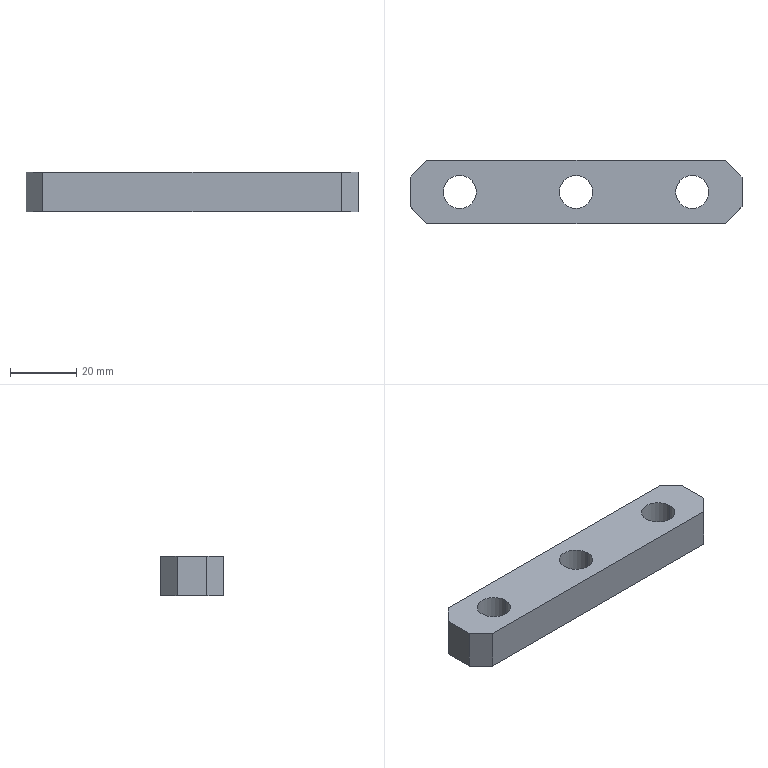Part | STEP file | J453-EBZ05-10-00 | 1 solid | 16 faces | box 100 x 19 x 12 mm | volume 19373 mm3 | plane 10 | cylinder 6 | commonest cylinder face diameters 10 x6
STEP:
#1=CARTESIAN_POINT('',(0.,0.,0.));
#2=DIRECTION('',(0.,0.,1.));
#3=DIRECTION('',(1.,0.,0.));
#4=AXIS2_PLACEMENT_3D('',#1,#2,#3);
#5=CARTESIAN_POINT('',(80.,10.,12.));
#6=VERTEX_POINT('',#5);
#7=CARTESIAN_POINT('',(80.,10.,0.));
#8=VERTEX_POINT('',#7);
#9=CARTESIAN_POINT('',(80.,10.,12.));
#10=DIRECTION('',(0.,0.,-1.));
#11=VECTOR('',#10,1.);
#12=LINE('',#9,#11);
#13=CARTESIAN_POINT('',(85.,10.,12.));
#14=DIRECTION('',(0.,0.,-1.));
#15=DIRECTION('',(-1.,0.,0.));
#16=AXIS2_PLACEMENT_3D('',#13,#14,#15);
#17=CYLINDRICAL_SURFACE('',#16,5.);
#18=CARTESIAN_POINT('',(6.283,0.));
#19=DIRECTION('',(0.,1.));
#20=VECTOR('',#19,1.);
#21=LINE('',#18,#20);
#22=(GEOMETRIC_REPRESENTATION_CONTEXT(2)PARAMETRIC_REPRESENTATION_CONTEXT()REPRESENTATION_CONTEXT('',''));
#23=DEFINITIONAL_REPRESENTATION('',(#21),#22);
#24=PCURVE('',#17,#23);
#25=CARTESIAN_POINT('',(85.,10.,12.));
#26=DIRECTION('',(0.,0.,-1.));
#27=DIRECTION('',(-1.,0.,0.));
#28=AXIS2_PLACEMENT_3D('',#25,#26,#27);
#29=CYLINDRICAL_SURFACE('',#28,5.);
#30=CARTESIAN_POINT('',(0.,0.));
#31=DIRECTION('',(0.,1.));
#32=VECTOR('',#31,1.);
#33=LINE('',#30,#32);
#34=(GEOMETRIC_REPRESENTATION_CONTEXT(2)PARAMETRIC_REPRESENTATION_CONTEXT()REPRESENTATION_CONTEXT('',''));
#35=DEFINITIONAL_REPRESENTATION('',(#33),#34);
#36=PCURVE('',#29,#35);
#37=SURFACE_CURVE('',#12,(#24,#36),.PCURVE_S1.);
#38=EDGE_CURVE('',#6,#8,#37,.T.);
#39=ORIENTED_EDGE('',*,*,#38,.T.);
#40=CARTESIAN_POINT('',(90.,10.,0.));
#41=VERTEX_POINT('',#40);
#42=CARTESIAN_POINT('',(85.,10.,0.));
#43=DIRECTION('',(0.,0.,1.));
#44=DIRECTION('',(1.,0.,0.));
#45=AXIS2_PLACEMENT_3D('',#42,#43,#44);
#46=CIRCLE('',#45,5.);
#47=CARTESIAN_POINT('',(9.425,12.));
#48=DIRECTION('',(-1.,0.));
#49=VECTOR('',#48,1.);
#50=LINE('',#47,#49);
#51=(GEOMETRIC_REPRESENTATION_CONTEXT(2)PARAMETRIC_REPRESENTATION_CONTEXT()REPRESENTATION_CONTEXT('',''));
#52=DEFINITIONAL_REPRESENTATION('',(#50),#51);
#53=PCURVE('',#17,#52);
#54=CARTESIAN_POINT('',(50.,10.,0.00000001));
#55=DIRECTION('',(0.,0.,-1.));
#56=DIRECTION('',(0.,-1.,0.));
#57=AXIS2_PLACEMENT_3D('',#54,#55,#56);
#58=PLANE('',#57);
#59=CARTESIAN_POINT('',(0.,-40.));
#60=CARTESIAN_POINT('',(-8.66,-40.));
#61=CARTESIAN_POINT('',(-4.33,-32.5));
#62=CARTESIAN_POINT('',(0.,-25.));
#63=CARTESIAN_POINT('',(4.33,-32.5));
#64=CARTESIAN_POINT('',(8.66,-40.));
#65=CARTESIAN_POINT('',(0.,-40.));
#66=(BOUNDED_CURVE()B_SPLINE_CURVE(2,(#59,#60,#61,#62,#63,#64,#65),.UNSPECIFIED.,.T.,.F.)B_SPLINE_CURVE_WITH_KNOTS((1,2,2,2,2,1),(-2.094,0.,2.094,4.189,6.283,8.378),.UNSPECIFIED.)CURVE()GEOMETRIC_REPRESENTATION_ITEM()RATIONAL_B_SPLINE_CURVE((1.,0.5,1.,0.5,1.,0.5,1.))REPRESENTATION_ITEM(''));
#67=(GEOMETRIC_REPRESENTATION_CONTEXT(2)PARAMETRIC_REPRESENTATION_CONTEXT()REPRESENTATION_CONTEXT('',''));
#68=DEFINITIONAL_REPRESENTATION('',(#66),#67);
#69=PCURVE('',#58,#68);
#70=SURFACE_CURVE('',#46,(#53,#69),.PCURVE_S1.);
#71=EDGE_CURVE('',#8,#41,#70,.T.);
#72=ORIENTED_EDGE('',*,*,#71,.T.);
#73=CARTESIAN_POINT('',(90.,10.,12.));
#74=VERTEX_POINT('',#73);
#75=CARTESIAN_POINT('',(90.,10.,12.));
#76=DIRECTION('',(0.,0.,-1.));
#77=VECTOR('',#76,1.);
#78=LINE('',#75,#77);
#79=CARTESIAN_POINT('',(3.142,0.));
#80=DIRECTION('',(0.,1.));
#81=VECTOR('',#80,1.);
#82=LINE('',#79,#81);
#83=(GEOMETRIC_REPRESENTATION_CONTEXT(2)PARAMETRIC_REPRESENTATION_CONTEXT()REPRESENTATION_CONTEXT('',''));
#84=DEFINITIONAL_REPRESENTATION('',(#82),#83);
#85=PCURVE('',#17,#84);
#86=CARTESIAN_POINT('',(3.142,0.));
#87=DIRECTION('',(0.,1.));
#88=VECTOR('',#87,1.);
#89=LINE('',#86,#88);
#90=(GEOMETRIC_REPRESENTATION_CONTEXT(2)PARAMETRIC_REPRESENTATION_CONTEXT()REPRESENTATION_CONTEXT('',''));
#91=DEFINITIONAL_REPRESENTATION('',(#89),#90);
#92=PCURVE('',#29,#91);
#93=SURFACE_CURVE('',#78,(#85,#92),.PCURVE_S1.);
#94=EDGE_CURVE('',#74,#41,#93,.T.);
#95=ORIENTED_EDGE('',*,*,#94,.F.);
#96=CARTESIAN_POINT('',(85.,10.,12.));
#97=DIRECTION('',(0.,0.,-1.));
#98=DIRECTION('',(-1.,0.,0.));
#99=AXIS2_PLACEMENT_3D('',#96,#97,#98);
#100=CIRCLE('',#99,5.);
#101=CARTESIAN_POINT('',(0.,0.));
#102=DIRECTION('',(1.,0.));
#103=VECTOR('',#102,1.);
#104=LINE('',#101,#103);
#105=(GEOMETRIC_REPRESENTATION_CONTEXT(2)PARAMETRIC_REPRESENTATION_CONTEXT()REPRESENTATION_CONTEXT('',''));
#106=DEFINITIONAL_REPRESENTATION('',(#104),#105);
#107=PCURVE('',#17,#106);
#108=CARTESIAN_POINT('',(50.,10.,12.));
#109=DIRECTION('',(0.,0.,1.));
#110=DIRECTION('',(0.,1.,0.));
#111=AXIS2_PLACEMENT_3D('',#108,#109,#110);
#112=PLANE('',#111);
#113=CARTESIAN_POINT('',(0.,-30.));
#114=CARTESIAN_POINT('',(8.66,-30.));
#115=CARTESIAN_POINT('',(4.33,-37.5));
#116=CARTESIAN_POINT('',(0.,-45.));
#117=CARTESIAN_POINT('',(-4.33,-37.5));
#118=CARTESIAN_POINT('',(-8.66,-30.));
#119=CARTESIAN_POINT('',(0.,-30.));
#120=(BOUNDED_CURVE()B_SPLINE_CURVE(2,(#113,#114,#115,#116,#117,#118,#119),.UNSPECIFIED.,.T.,.F.)B_SPLINE_CURVE_WITH_KNOTS((1,2,2,2,2,1),(-2.094,0.,2.094,4.189,6.283,8.378),.UNSPECIFIED.)CURVE()GEOMETRIC_REPRESENTATION_ITEM()RATIONAL_B_SPLINE_CURVE((1.,0.5,1.,0.5,1.,0.5,1.))REPRESENTATION_ITEM(''));
#121=(GEOMETRIC_REPRESENTATION_CONTEXT(2)PARAMETRIC_REPRESENTATION_CONTEXT()REPRESENTATION_CONTEXT('',''));
#122=DEFINITIONAL_REPRESENTATION('',(#120),#121);
#123=PCURVE('',#112,#122);
#124=SURFACE_CURVE('',#100,(#107,#123),.PCURVE_S1.);
#125=EDGE_CURVE('',#74,#6,#124,.T.);
#126=ORIENTED_EDGE('',*,*,#125,.T.);
#127=EDGE_LOOP('',(#39,#72,#95,#126));
#128=FACE_BOUND('',#127,.F.);
#129=ADVANCED_FACE('',(#128),#17,.F.);
#130=CARTESIAN_POINT('',(45.,10.,12.));
#131=VERTEX_POINT('',#130);
#132=CARTESIAN_POINT('',(45.,10.,0.));
#133=VERTEX_POINT('',#132);
#134=CARTESIAN_POINT('',(45.,10.,12.));
#135=DIRECTION('',(0.,0.,-1.));
#136=VECTOR('',#135,1.);
#137=LINE('',#134,#136);
#138=CARTESIAN_POINT('',(50.,10.,12.));
#139=DIRECTION('',(0.,0.,-1.));
#140=DIRECTION('',(-1.,0.,0.));
#141=AXIS2_PLACEMENT_3D('',#138,#139,#140);
#142=CYLINDRICAL_SURFACE('',#141,5.);
#143=CARTESIAN_POINT('',(6.283,0.));
#144=DIRECTION('',(0.,1.));
#145=VECTOR('',#144,1.);
#146=LINE('',#143,#145);
#147=(GEOMETRIC_REPRESENTATION_CONTEXT(2)PARAMETRIC_REPRESENTATION_CONTEXT()REPRESENTATION_CONTEXT('',''));
#148=DEFINITIONAL_REPRESENTATION('',(#146),#147);
#149=PCURVE('',#142,#148);
#150=CARTESIAN_POINT('',(50.,10.,12.));
#151=DIRECTION('',(0.,0.,-1.));
#152=DIRECTION('',(-1.,0.,0.));
#153=AXIS2_PLACEMENT_3D('',#150,#151,#152);
#154=CYLINDRICAL_SURFACE('',#153,5.);
#155=CARTESIAN_POINT('',(0.,0.));
#156=DIRECTION('',(0.,1.));
#157=VECTOR('',#156,1.);
#158=LINE('',#155,#157);
#159=(GEOMETRIC_REPRESENTATION_CONTEXT(2)PARAMETRIC_REPRESENTATION_CONTEXT()REPRESENTATION_CONTEXT('',''));
#160=DEFINITIONAL_REPRESENTATION('',(#158),#159);
#161=PCURVE('',#154,#160);
#162=SURFACE_CURVE('',#137,(#149,#161),.PCURVE_S1.);
#163=EDGE_CURVE('',#131,#133,#162,.T.);
#164=ORIENTED_EDGE('',*,*,#163,.T.);
#165=CARTESIAN_POINT('',(55.,10.,0.));
#166=VERTEX_POINT('',#165);
#167=CARTESIAN_POINT('',(50.,10.,0.));
#168=DIRECTION('',(0.,0.,1.));
#169=DIRECTION('',(1.,0.,0.));
#170=AXIS2_PLACEMENT_3D('',#167,#168,#169);
#171=CIRCLE('',#170,5.);
#172=CARTESIAN_POINT('',(9.425,12.));
#173=DIRECTION('',(-1.,0.));
#174=VECTOR('',#173,1.);
#175=LINE('',#172,#174);
#176=(GEOMETRIC_REPRESENTATION_CONTEXT(2)PARAMETRIC_REPRESENTATION_CONTEXT()REPRESENTATION_CONTEXT('',''));
#177=DEFINITIONAL_REPRESENTATION('',(#175),#176);
#178=PCURVE('',#142,#177);
#179=CARTESIAN_POINT('',(0.,-5.));
#180=CARTESIAN_POINT('',(-8.66,-5.));
#181=CARTESIAN_POINT('',(-4.33,2.5));
#182=CARTESIAN_POINT('',(0.,10.));
#183=CARTESIAN_POINT('',(4.33,2.5));
#184=CARTESIAN_POINT('',(8.66,-5.));
#185=CARTESIAN_POINT('',(0.,-5.));
#186=(BOUNDED_CURVE()B_SPLINE_CURVE(2,(#179,#180,#181,#182,#183,#184,#185),.UNSPECIFIED.,.T.,.F.)B_SPLINE_CURVE_WITH_KNOTS((1,2,2,2,2,1),(-2.094,0.,2.094,4.189,6.283,8.378),.UNSPECIFIED.)CURVE()GEOMETRIC_REPRESENTATION_ITEM()RATIONAL_B_SPLINE_CURVE((1.,0.5,1.,0.5,1.,0.5,1.))REPRESENTATION_ITEM(''));
#187=(GEOMETRIC_REPRESENTATION_CONTEXT(2)PARAMETRIC_REPRESENTATION_CONTEXT()REPRESENTATION_CONTEXT('',''));
#188=DEFINITIONAL_REPRESENTATION('',(#186),#187);
#189=PCURVE('',#58,#188);
#190=SURFACE_CURVE('',#171,(#178,#189),.PCURVE_S1.);
#191=EDGE_CURVE('',#133,#166,#190,.T.);
#192=ORIENTED_EDGE('',*,*,#191,.T.);
#193=CARTESIAN_POINT('',(55.,10.,12.));
#194=VERTEX_POINT('',#193);
#195=CARTESIAN_POINT('',(55.,10.,12.));
#196=DIRECTION('',(0.,0.,-1.));
#197=VECTOR('',#196,1.);
#198=LINE('',#195,#197);
#199=CARTESIAN_POINT('',(3.142,0.));
#200=DIRECTION('',(0.,1.));
#201=VECTOR('',#200,1.);
#202=LINE('',#199,#201);
#203=(GEOMETRIC_REPRESENTATION_CONTEXT(2)PARAMETRIC_REPRESENTATION_CONTEXT()REPRESENTATION_CONTEXT('',''));
#204=DEFINITIONAL_REPRESENTATION('',(#202),#203);
#205=PCURVE('',#142,#204);
#206=CARTESIAN_POINT('',(3.142,0.));
#207=DIRECTION('',(0.,1.));
#208=VECTOR('',#207,1.);
#209=LINE('',#206,#208);
#210=(GEOMETRIC_REPRESENTATION_CONTEXT(2)PARAMETRIC_REPRESENTATION_CONTEXT()REPRESENTATION_CONTEXT('',''));
#211=DEFINITIONAL_REPRESENTATION('',(#209),#210);
#212=PCURVE('',#154,#211);
#213=SURFACE_CURVE('',#198,(#205,#212),.PCURVE_S1.);
#214=EDGE_CURVE('',#194,#166,#213,.T.);
#215=ORIENTED_EDGE('',*,*,#214,.F.);
#216=CARTESIAN_POINT('',(50.,10.,12.));
#217=DIRECTION('',(0.,0.,-1.));
#218=DIRECTION('',(-1.,0.,0.));
#219=AXIS2_PLACEMENT_3D('',#216,#217,#218);
#220=CIRCLE('',#219,5.);
#221=CARTESIAN_POINT('',(0.,0.));
#222=DIRECTION('',(1.,0.));
#223=VECTOR('',#222,1.);
#224=LINE('',#221,#223);
#225=(GEOMETRIC_REPRESENTATION_CONTEXT(2)PARAMETRIC_REPRESENTATION_CONTEXT()REPRESENTATION_CONTEXT('',''));
#226=DEFINITIONAL_REPRESENTATION('',(#224),#225);
#227=PCURVE('',#142,#226);
#228=CARTESIAN_POINT('',(0.,5.));
#229=CARTESIAN_POINT('',(8.66,5.));
#230=CARTESIAN_POINT('',(4.33,-2.5));
#231=CARTESIAN_POINT('',(0.,-10.));
#232=CARTESIAN_POINT('',(-4.33,-2.5));
#233=CARTESIAN_POINT('',(-8.66,5.));
#234=CARTESIAN_POINT('',(0.,5.));
#235=(BOUNDED_CURVE()B_SPLINE_CURVE(2,(#228,#229,#230,#231,#232,#233,#234),.UNSPECIFIED.,.T.,.F.)B_SPLINE_CURVE_WITH_KNOTS((1,2,2,2,2,1),(-2.094,0.,2.094,4.189,6.283,8.378),.UNSPECIFIED.)CURVE()GEOMETRIC_REPRESENTATION_ITEM()RATIONAL_B_SPLINE_CURVE((1.,0.5,1.,0.5,1.,0.5,1.))REPRESENTATION_ITEM(''));
#236=(GEOMETRIC_REPRESENTATION_CONTEXT(2)PARAMETRIC_REPRESENTATION_CONTEXT()REPRESENTATION_CONTEXT('',''));
#237=DEFINITIONAL_REPRESENTATION('',(#235),#236);
#238=PCURVE('',#112,#237);
#239=SURFACE_CURVE('',#220,(#227,#238),.PCURVE_S1.);
#240=EDGE_CURVE('',#194,#131,#239,.T.);
#241=ORIENTED_EDGE('',*,*,#240,.T.);
#242=EDGE_LOOP('',(#164,#192,#215,#241));
#243=FACE_BOUND('',#242,.F.);
#244=ADVANCED_FACE('',(#243),#142,.F.);
#245=CARTESIAN_POINT('',(10.,10.,12.));
#246=VERTEX_POINT('',#245);
#247=CARTESIAN_POINT('',(10.,10.,0.));
#248=VERTEX_POINT('',#247);
#249=CARTESIAN_POINT('',(10.,10.,12.));
#250=DIRECTION('',(0.,0.,-1.));
#251=VECTOR('',#250,1.);
#252=LINE('',#249,#251);
#253=CARTESIAN_POINT('',(15.,10.,12.));
#254=DIRECTION('',(0.,0.,-1.));
#255=DIRECTION('',(-1.,0.,0.));
#256=AXIS2_PLACEMENT_3D('',#253,#254,#255);
#257=CYLINDRICAL_SURFACE('',#256,5.);
#258=CARTESIAN_POINT('',(6.283,0.));
#259=DIRECTION('',(0.,1.));
#260=VECTOR('',#259,1.);
#261=LINE('',#258,#260);
#262=(GEOMETRIC_REPRESENTATION_CONTEXT(2)PARAMETRIC_REPRESENTATION_CONTEXT()REPRESENTATION_CONTEXT('',''));
#263=DEFINITIONAL_REPRESENTATION('',(#261),#262);
#264=PCURVE('',#257,#263);
#265=CARTESIAN_POINT('',(15.,10.,12.));
#266=DIRECTION('',(0.,0.,-1.));
#267=DIRECTION('',(-1.,0.,0.));
#268=AXIS2_PLACEMENT_3D('',#265,#266,#267);
#269=CYLINDRICAL_SURFACE('',#268,5.);
#270=CARTESIAN_POINT('',(0.,0.));
#271=DIRECTION('',(0.,1.));
#272=VECTOR('',#271,1.);
#273=LINE('',#270,#272);
#274=(GEOMETRIC_REPRESENTATION_CONTEXT(2)PARAMETRIC_REPRESENTATION_CONTEXT()REPRESENTATION_CONTEXT('',''));
#275=DEFINITIONAL_REPRESENTATION('',(#273),#274);
#276=PCURVE('',#269,#275);
#277=SURFACE_CURVE('',#252,(#264,#276),.PCURVE_S1.);
#278=EDGE_CURVE('',#246,#248,#277,.T.);
#279=ORIENTED_EDGE('',*,*,#278,.T.);
#280=CARTESIAN_POINT('',(20.,10.,0.));
#281=VERTEX_POINT('',#280);
#282=CARTESIAN_POINT('',(15.,10.,0.));
#283=DIRECTION('',(0.,0.,1.));
#284=DIRECTION('',(1.,0.,0.));
#285=AXIS2_PLACEMENT_3D('',#282,#283,#284);
#286=CIRCLE('',#285,5.);
#287=CARTESIAN_POINT('',(9.425,12.));
#288=DIRECTION('',(-1.,0.));
#289=VECTOR('',#288,1.);
#290=LINE('',#287,#289);
#291=(GEOMETRIC_REPRESENTATION_CONTEXT(2)PARAMETRIC_REPRESENTATION_CONTEXT()REPRESENTATION_CONTEXT('',''));
#292=DEFINITIONAL_REPRESENTATION('',(#290),#291);
#293=PCURVE('',#257,#292);
#294=CARTESIAN_POINT('',(0.,30.));
#295=CARTESIAN_POINT('',(-8.66,30.));
#296=CARTESIAN_POINT('',(-4.33,37.5));
#297=CARTESIAN_POINT('',(0.,45.));
#298=CARTESIAN_POINT('',(4.33,37.5));
#299=CARTESIAN_POINT('',(8.66,30.));
#300=CARTESIAN_POINT('',(0.,30.));
#301=(BOUNDED_CURVE()B_SPLINE_CURVE(2,(#294,#295,#296,#297,#298,#299,#300),.UNSPECIFIED.,.T.,.F.)B_SPLINE_CURVE_WITH_KNOTS((1,2,2,2,2,1),(-2.094,0.,2.094,4.189,6.283,8.378),.UNSPECIFIED.)CURVE()GEOMETRIC_REPRESENTATION_ITEM()RATIONAL_B_SPLINE_CURVE((1.,0.5,1.,0.5,1.,0.5,1.))REPRESENTATION_ITEM(''));
#302=(GEOMETRIC_REPRESENTATION_CONTEXT(2)PARAMETRIC_REPRESENTATION_CONTEXT()REPRESENTATION_CONTEXT('',''));
#303=DEFINITIONAL_REPRESENTATION('',(#301),#302);
#304=PCURVE('',#58,#303);
#305=SURFACE_CURVE('',#286,(#293,#304),.PCURVE_S1.);
#306=EDGE_CURVE('',#248,#281,#305,.T.);
#307=ORIENTED_EDGE('',*,*,#306,.T.);
#308=CARTESIAN_POINT('',(20.,10.,12.));
#309=VERTEX_POINT('',#308);
#310=CARTESIAN_POINT('',(20.,10.,12.));
#311=DIRECTION('',(0.,0.,-1.));
#312=VECTOR('',#311,1.);
#313=LINE('',#310,#312);
#314=CARTESIAN_POINT('',(3.142,0.));
#315=DIRECTION('',(0.,1.));
#316=VECTOR('',#315,1.);
#317=LINE('',#314,#316);
#318=(GEOMETRIC_REPRESENTATION_CONTEXT(2)PARAMETRIC_REPRESENTATION_CONTEXT()REPRESENTATION_CONTEXT('',''));
#319=DEFINITIONAL_REPRESENTATION('',(#317),#318);
#320=PCURVE('',#257,#319);
#321=CARTESIAN_POINT('',(3.142,0.));
#322=DIRECTION('',(0.,1.));
#323=VECTOR('',#322,1.);
#324=LINE('',#321,#323);
#325=(GEOMETRIC_REPRESENTATION_CONTEXT(2)PARAMETRIC_REPRESENTATION_CONTEXT()REPRESENTATION_CONTEXT('',''));
#326=DEFINITIONAL_REPRESENTATION('',(#324),#325);
#327=PCURVE('',#269,#326);
#328=SURFACE_CURVE('',#313,(#320,#327),.PCURVE_S1.);
#329=EDGE_CURVE('',#309,#281,#328,.T.);
#330=ORIENTED_EDGE('',*,*,#329,.F.);
#331=CARTESIAN_POINT('',(15.,10.,12.));
#332=DIRECTION('',(0.,0.,-1.));
#333=DIRECTION('',(-1.,0.,0.));
#334=AXIS2_PLACEMENT_3D('',#331,#332,#333);
#335=CIRCLE('',#334,5.);
#336=CARTESIAN_POINT('',(0.,0.));
#337=DIRECTION('',(1.,0.));
#338=VECTOR('',#337,1.);
#339=LINE('',#336,#338);
#340=(GEOMETRIC_REPRESENTATION_CONTEXT(2)PARAMETRIC_REPRESENTATION_CONTEXT()REPRESENTATION_CONTEXT('',''));
#341=DEFINITIONAL_REPRESENTATION('',(#339),#340);
#342=PCURVE('',#257,#341);
#343=CARTESIAN_POINT('',(0.,40.));
#344=CARTESIAN_POINT('',(8.66,40.));
#345=CARTESIAN_POINT('',(4.33,32.5));
#346=CARTESIAN_POINT('',(0.,25.));
#347=CARTESIAN_POINT('',(-4.33,32.5));
#348=CARTESIAN_POINT('',(-8.66,40.));
#349=CARTESIAN_POINT('',(0.,40.));
#350=(BOUNDED_CURVE()B_SPLINE_CURVE(2,(#343,#344,#345,#346,#347,#348,#349),.UNSPECIFIED.,.T.,.F.)B_SPLINE_CURVE_WITH_KNOTS((1,2,2,2,2,1),(-2.094,0.,2.094,4.189,6.283,8.378),.UNSPECIFIED.)CURVE()GEOMETRIC_REPRESENTATION_ITEM()RATIONAL_B_SPLINE_CURVE((1.,0.5,1.,0.5,1.,0.5,1.))REPRESENTATION_ITEM(''));
#351=(GEOMETRIC_REPRESENTATION_CONTEXT(2)PARAMETRIC_REPRESENTATION_CONTEXT()REPRESENTATION_CONTEXT('',''));
#352=DEFINITIONAL_REPRESENTATION('',(#350),#351);
#353=PCURVE('',#112,#352);
#354=SURFACE_CURVE('',#335,(#342,#353),.PCURVE_S1.);
#355=EDGE_CURVE('',#309,#246,#354,.T.);
#356=ORIENTED_EDGE('',*,*,#355,.T.);
#357=EDGE_LOOP('',(#279,#307,#330,#356));
#358=FACE_BOUND('',#357,.F.);
#359=ADVANCED_FACE('',(#358),#257,.F.);
#360=CARTESIAN_POINT('',(85.,10.,12.));
#361=DIRECTION('',(0.,0.,-1.));
#362=DIRECTION('',(-1.,0.,0.));
#363=AXIS2_PLACEMENT_3D('',#360,#361,#362);
#364=CIRCLE('',#363,5.);
#365=CARTESIAN_POINT('',(0.,-30.));
#366=CARTESIAN_POINT('',(8.66,-30.));
#367=CARTESIAN_POINT('',(4.33,-37.5));
#368=CARTESIAN_POINT('',(0.,-45.));
#369=CARTESIAN_POINT('',(-4.33,-37.5));
#370=CARTESIAN_POINT('',(-8.66,-30.));
#371=CARTESIAN_POINT('',(0.,-30.));
#372=(BOUNDED_CURVE()B_SPLINE_CURVE(2,(#365,#366,#367,#368,#369,#370,#371),.UNSPECIFIED.,.T.,.F.)B_SPLINE_CURVE_WITH_KNOTS((1,2,2,2,2,1),(-2.094,0.,2.094,4.189,6.283,8.378),.UNSPECIFIED.)CURVE()GEOMETRIC_REPRESENTATION_ITEM()RATIONAL_B_SPLINE_CURVE((1.,0.5,1.,0.5,1.,0.5,1.))REPRESENTATION_ITEM(''));
#373=(GEOMETRIC_REPRESENTATION_CONTEXT(2)PARAMETRIC_REPRESENTATION_CONTEXT()REPRESENTATION_CONTEXT('',''));
#374=DEFINITIONAL_REPRESENTATION('',(#372),#373);
#375=PCURVE('',#112,#374);
#376=CARTESIAN_POINT('',(0.,0.));
#377=DIRECTION('',(1.,0.));
#378=VECTOR('',#377,1.);
#379=LINE('',#376,#378);
#380=(GEOMETRIC_REPRESENTATION_CONTEXT(2)PARAMETRIC_REPRESENTATION_CONTEXT()REPRESENTATION_CONTEXT('',''));
#381=DEFINITIONAL_REPRESENTATION('',(#379),#380);
#382=PCURVE('',#29,#381);
#383=SURFACE_CURVE('',#364,(#375,#382),.PCURVE_S1.);
#384=EDGE_CURVE('',#6,#74,#383,.T.);
#385=ORIENTED_EDGE('',*,*,#384,.T.);
#386=ORIENTED_EDGE('',*,*,#125,.T.);
#387=EDGE_LOOP('',(#385,#386));
#388=FACE_BOUND('',#387,.T.);
#389=CARTESIAN_POINT('',(50.,10.,12.));
#390=DIRECTION('',(0.,0.,-1.));
#391=DIRECTION('',(-1.,0.,0.));
#392=AXIS2_PLACEMENT_3D('',#389,#390,#391);
#393=CIRCLE('',#392,5.);
#394=CARTESIAN_POINT('',(0.,5.));
#395=CARTESIAN_POINT('',(8.66,5.));
#396=CARTESIAN_POINT('',(4.33,-2.5));
#397=CARTESIAN_POINT('',(0.,-10.));
#398=CARTESIAN_POINT('',(-4.33,-2.5));
#399=CARTESIAN_POINT('',(-8.66,5.));
#400=CARTESIAN_POINT('',(0.,5.));
#401=(BOUNDED_CURVE()B_SPLINE_CURVE(2,(#394,#395,#396,#397,#398,#399,#400),.UNSPECIFIED.,.T.,.F.)B_SPLINE_CURVE_WITH_KNOTS((1,2,2,2,2,1),(-2.094,0.,2.094,4.189,6.283,8.378),.UNSPECIFIED.)CURVE()GEOMETRIC_REPRESENTATION_ITEM()RATIONAL_B_SPLINE_CURVE((1.,0.5,1.,0.5,1.,0.5,1.))REPRESENTATION_ITEM(''));
#402=(GEOMETRIC_REPRESENTATION_CONTEXT(2)PARAMETRIC_REPRESENTATION_CONTEXT()REPRESENTATION_CONTEXT('',''));
#403=DEFINITIONAL_REPRESENTATION('',(#401),#402);
#404=PCURVE('',#112,#403);
#405=CARTESIAN_POINT('',(0.,0.));
#406=DIRECTION('',(1.,0.));
#407=VECTOR('',#406,1.);
#408=LINE('',#405,#407);
#409=(GEOMETRIC_REPRESENTATION_CONTEXT(2)PARAMETRIC_REPRESENTATION_CONTEXT()REPRESENTATION_CONTEXT('',''));
#410=DEFINITIONAL_REPRESENTATION('',(#408),#409);
#411=PCURVE('',#154,#410);
#412=SURFACE_CURVE('',#393,(#404,#411),.PCURVE_S1.);
#413=EDGE_CURVE('',#131,#194,#412,.T.);
#414=ORIENTED_EDGE('',*,*,#413,.T.);
#415=ORIENTED_EDGE('',*,*,#240,.T.);
#416=EDGE_LOOP('',(#414,#415));
#417=FACE_BOUND('',#416,.T.);
#418=CARTESIAN_POINT('',(15.,10.,12.));
#419=DIRECTION('',(0.,0.,-1.));
#420=DIRECTION('',(-1.,0.,0.));
#421=AXIS2_PLACEMENT_3D('',#418,#419,#420);
#422=CIRCLE('',#421,5.);
#423=CARTESIAN_POINT('',(0.,40.));
#424=CARTESIAN_POINT('',(8.66,40.));
#425=CARTESIAN_POINT('',(4.33,32.5));
#426=CARTESIAN_POINT('',(0.,25.));
#427=CARTESIAN_POINT('',(-4.33,32.5));
#428=CARTESIAN_POINT('',(-8.66,40.));
#429=CARTESIAN_POINT('',(0.,40.));
#430=(BOUNDED_CURVE()B_SPLINE_CURVE(2,(#423,#424,#425,#426,#427,#428,#429),.UNSPECIFIED.,.T.,.F.)B_SPLINE_CURVE_WITH_KNOTS((1,2,2,2,2,1),(-2.094,0.,2.094,4.189,6.283,8.378),.UNSPECIFIED.)CURVE()GEOMETRIC_REPRESENTATION_ITEM()RATIONAL_B_SPLINE_CURVE((1.,0.5,1.,0.5,1.,0.5,1.))REPRESENTATION_ITEM(''));
#431=(GEOMETRIC_REPRESENTATION_CONTEXT(2)PARAMETRIC_REPRESENTATION_CONTEXT()REPRESENTATION_CONTEXT('',''));
#432=DEFINITIONAL_REPRESENTATION('',(#430),#431);
#433=PCURVE('',#112,#432);
#434=CARTESIAN_POINT('',(0.,0.));
#435=DIRECTION('',(1.,0.));
#436=VECTOR('',#435,1.);
#437=LINE('',#434,#436);
#438=(GEOMETRIC_REPRESENTATION_CONTEXT(2)PARAMETRIC_REPRESENTATION_CONTEXT()REPRESENTATION_CONTEXT('',''));
#439=DEFINITIONAL_REPRESENTATION('',(#437),#438);
#440=PCURVE('',#269,#439);
#441=SURFACE_CURVE('',#422,(#433,#440),.PCURVE_S1.);
#442=EDGE_CURVE('',#246,#309,#441,.T.);
#443=ORIENTED_EDGE('',*,*,#442,.T.);
#444=ORIENTED_EDGE('',*,*,#355,.T.);
#445=EDGE_LOOP('',(#443,#444));
#446=FACE_BOUND('',#445,.T.);
#447=CARTESIAN_POINT('',(5.,19.5,12.));
#448=VERTEX_POINT('',#447);
#449=CARTESIAN_POINT('',(95.,19.5,12.));
#450=VERTEX_POINT('',#449);
#451=CARTESIAN_POINT('',(50.,19.5,12.));
#452=DIRECTION('',(1.,0.,0.));
#453=VECTOR('',#452,1.);
#454=LINE('',#451,#453);
#455=CARTESIAN_POINT('',(9.5,0.));
#456=DIRECTION('',(0.,-1.));
#457=VECTOR('',#456,1.);
#458=LINE('',#455,#457);
#459=(GEOMETRIC_REPRESENTATION_CONTEXT(2)PARAMETRIC_REPRESENTATION_CONTEXT()REPRESENTATION_CONTEXT('',''));
#460=DEFINITIONAL_REPRESENTATION('',(#458),#459);
#461=PCURVE('',#112,#460);
#462=CARTESIAN_POINT('',(50.,19.5,0.00000001));
#463=DIRECTION('',(0.,1.,0.));
#464=DIRECTION('',(0.,0.,-1.));
#465=AXIS2_PLACEMENT_3D('',#462,#463,#464);
#466=PLANE('',#465);
#467=CARTESIAN_POINT('',(-12.,0.));
#468=DIRECTION('',(0.,-1.));
#469=VECTOR('',#468,1.);
#470=LINE('',#467,#469);
#471=(GEOMETRIC_REPRESENTATION_CONTEXT(2)PARAMETRIC_REPRESENTATION_CONTEXT()REPRESENTATION_CONTEXT('',''));
#472=DEFINITIONAL_REPRESENTATION('',(#470),#471);
#473=PCURVE('',#466,#472);
#474=SURFACE_CURVE('',#454,(#461,#473),.PCURVE_S1.);
#475=EDGE_CURVE('',#448,#450,#474,.T.);
#476=ORIENTED_EDGE('',*,*,#475,.F.);
#477=CARTESIAN_POINT('',(0.,14.5,12.));
#478=VERTEX_POINT('',#477);
#479=CARTESIAN_POINT('',(22.75,37.25,12.));
#480=DIRECTION('',(-0.7071,-0.7071,0.));
#481=VECTOR('',#480,1.);
#482=LINE('',#479,#481);
#483=CARTESIAN_POINT('',(27.25,27.25));
#484=DIRECTION('',(-0.7071,0.7071));
#485=VECTOR('',#484,1.);
#486=LINE('',#483,#485);
#487=(GEOMETRIC_REPRESENTATION_CONTEXT(2)PARAMETRIC_REPRESENTATION_CONTEXT()REPRESENTATION_CONTEXT('',''));
#488=DEFINITIONAL_REPRESENTATION('',(#486),#487);
#489=PCURVE('',#112,#488);
#490=CARTESIAN_POINT('',(5.,19.5,0.00000001));
#491=DIRECTION('',(0.7071,-0.7071,0.));
#492=DIRECTION('',(0.,0.,1.));
#493=AXIS2_PLACEMENT_3D('',#490,#491,#492);
#494=PLANE('',#493);
#495=CARTESIAN_POINT('',(12.,-25.102));
#496=DIRECTION('',(0.,1.));
#497=VECTOR('',#496,1.);
#498=LINE('',#495,#497);
#499=(GEOMETRIC_REPRESENTATION_CONTEXT(2)PARAMETRIC_REPRESENTATION_CONTEXT()REPRESENTATION_CONTEXT('',''));
#500=DEFINITIONAL_REPRESENTATION('',(#498),#499);
#501=PCURVE('',#494,#500);
#502=SURFACE_CURVE('',#482,(#489,#501),.PCURVE_S1.);
#503=EDGE_CURVE('',#448,#478,#502,.T.);
#504=ORIENTED_EDGE('',*,*,#503,.T.);
#505=CARTESIAN_POINT('',(0.,5.5,12.));
#506=VERTEX_POINT('',#505);
#507=CARTESIAN_POINT('',(0.,10.,12.));
#508=DIRECTION('',(0.,1.,0.));
#509=VECTOR('',#508,1.);
#510=LINE('',#507,#509);
#511=CARTESIAN_POINT('',(0.,50.));
#512=DIRECTION('',(1.,0.));
#513=VECTOR('',#512,1.);
#514=LINE('',#511,#513);
#515=(GEOMETRIC_REPRESENTATION_CONTEXT(2)PARAMETRIC_REPRESENTATION_CONTEXT()REPRESENTATION_CONTEXT('',''));
#516=DEFINITIONAL_REPRESENTATION('',(#514),#515);
#517=PCURVE('',#112,#516);
#518=CARTESIAN_POINT('',(0.,10.,0.00000001));
#519=DIRECTION('',(-1.,0.,0.));
#520=DIRECTION('',(0.,0.,1.));
#521=AXIS2_PLACEMENT_3D('',#518,#519,#520);
#522=PLANE('',#521);
#523=CARTESIAN_POINT('',(12.,0.));
#524=DIRECTION('',(0.,1.));
#525=VECTOR('',#524,1.);
#526=LINE('',#523,#525);
#527=(GEOMETRIC_REPRESENTATION_CONTEXT(2)PARAMETRIC_REPRESENTATION_CONTEXT()REPRESENTATION_CONTEXT('',''));
#528=DEFINITIONAL_REPRESENTATION('',(#526),#527);
#529=PCURVE('',#522,#528);
#530=SURFACE_CURVE('',#510,(#517,#529),.PCURVE_S1.);
#531=EDGE_CURVE('',#506,#478,#530,.T.);
#532=ORIENTED_EDGE('',*,*,#531,.F.);
#533=CARTESIAN_POINT('',(5.,0.5,12.));
#534=VERTEX_POINT('',#533);
#535=CARTESIAN_POINT('',(22.75,-17.25,12.));
#536=DIRECTION('',(0.7071,-0.7071,0.));
#537=VECTOR('',#536,1.);
#538=LINE('',#535,#537);
#539=CARTESIAN_POINT('',(-27.25,27.25));
#540=DIRECTION('',(-0.7071,-0.7071));
#541=VECTOR('',#540,1.);
#542=LINE('',#539,#541);
#543=(GEOMETRIC_REPRESENTATION_CONTEXT(2)PARAMETRIC_REPRESENTATION_CONTEXT()REPRESENTATION_CONTEXT('',''));
#544=DEFINITIONAL_REPRESENTATION('',(#542),#543);
#545=PCURVE('',#112,#544);
#546=CARTESIAN_POINT('',(0.,5.5,0.00000001));
#547=DIRECTION('',(0.7071,0.7071,0.));
#548=DIRECTION('',(0.,0.,1.));
#549=AXIS2_PLACEMENT_3D('',#546,#547,#548);
#550=PLANE('',#549);
#551=CARTESIAN_POINT('',(12.,32.173));
#552=DIRECTION('',(0.,1.));
#553=VECTOR('',#552,1.);
#554=LINE('',#551,#553);
#555=(GEOMETRIC_REPRESENTATION_CONTEXT(2)PARAMETRIC_REPRESENTATION_CONTEXT()REPRESENTATION_CONTEXT('',''));
#556=DEFINITIONAL_REPRESENTATION('',(#554),#555);
#557=PCURVE('',#550,#556);
#558=SURFACE_CURVE('',#538,(#545,#557),.PCURVE_S1.);
#559=EDGE_CURVE('',#506,#534,#558,.T.);
#560=ORIENTED_EDGE('',*,*,#559,.T.);
#561=CARTESIAN_POINT('',(95.,0.5,12.));
#562=VERTEX_POINT('',#561);
#563=CARTESIAN_POINT('',(50.,0.5,12.));
#564=DIRECTION('',(-1.,0.,0.));
#565=VECTOR('',#564,1.);
#566=LINE('',#563,#565);
#567=CARTESIAN_POINT('',(-9.5,0.));
#568=DIRECTION('',(0.,1.));
#569=VECTOR('',#568,1.);
#570=LINE('',#567,#569);
#571=(GEOMETRIC_REPRESENTATION_CONTEXT(2)PARAMETRIC_REPRESENTATION_CONTEXT()REPRESENTATION_CONTEXT('',''));
#572=DEFINITIONAL_REPRESENTATION('',(#570),#571);
#573=PCURVE('',#112,#572);
#574=CARTESIAN_POINT('',(50.,0.5,0.00000001));
#575=DIRECTION('',(0.,-1.,0.));
#576=DIRECTION('',(0.,0.,1.));
#577=AXIS2_PLACEMENT_3D('',#574,#575,#576);
#578=PLANE('',#577);
#579=CARTESIAN_POINT('',(12.,0.));
#580=DIRECTION('',(0.,1.));
#581=VECTOR('',#580,1.);
#582=LINE('',#579,#581);
#583=(GEOMETRIC_REPRESENTATION_CONTEXT(2)PARAMETRIC_REPRESENTATION_CONTEXT()REPRESENTATION_CONTEXT('',''));
#584=DEFINITIONAL_REPRESENTATION('',(#582),#583);
#585=PCURVE('',#578,#584);
#586=SURFACE_CURVE('',#566,(#573,#585),.PCURVE_S1.);
#587=EDGE_CURVE('',#562,#534,#586,.T.);
#588=ORIENTED_EDGE('',*,*,#587,.F.);
#589=CARTESIAN_POINT('',(100.,5.5,12.));
#590=VERTEX_POINT('',#589);
#591=CARTESIAN_POINT('',(77.25,-17.25,12.));
#592=DIRECTION('',(0.7071,0.7071,0.));
#593=VECTOR('',#592,1.);
#594=LINE('',#591,#593);
#595=CARTESIAN_POINT('',(-27.25,-27.25));
#596=DIRECTION('',(0.7071,-0.7071));
#597=VECTOR('',#596,1.);
#598=LINE('',#595,#597);
#599=(GEOMETRIC_REPRESENTATION_CONTEXT(2)PARAMETRIC_REPRESENTATION_CONTEXT()REPRESENTATION_CONTEXT('',''));
#600=DEFINITIONAL_REPRESENTATION('',(#598),#599);
#601=PCURVE('',#112,#600);
#602=CARTESIAN_POINT('',(95.,0.5,0.00000001));
#603=DIRECTION('',(-0.7071,0.7071,0.));
#604=DIRECTION('',(0.,0.,1.));
#605=AXIS2_PLACEMENT_3D('',#602,#603,#604);
#606=PLANE('',#605);
#607=CARTESIAN_POINT('',(12.,-25.102));
#608=DIRECTION('',(0.,1.));
#609=VECTOR('',#608,1.);
#610=LINE('',#607,#609);
#611=(GEOMETRIC_REPRESENTATION_CONTEXT(2)PARAMETRIC_REPRESENTATION_CONTEXT()REPRESENTATION_CONTEXT('',''));
#612=DEFINITIONAL_REPRESENTATION('',(#610),#611);
#613=PCURVE('',#606,#612);
#614=SURFACE_CURVE('',#594,(#601,#613),.PCURVE_S1.);
#615=EDGE_CURVE('',#562,#590,#614,.T.);
#616=ORIENTED_EDGE('',*,*,#615,.T.);
#617=CARTESIAN_POINT('',(100.,14.5,12.));
#618=VERTEX_POINT('',#617);
#619=CARTESIAN_POINT('',(100.,10.,12.));
#620=DIRECTION('',(0.,-1.,0.));
#621=VECTOR('',#620,1.);
#622=LINE('',#619,#621);
#623=CARTESIAN_POINT('',(0.,-50.));
#624=DIRECTION('',(-1.,0.));
#625=VECTOR('',#624,1.);
#626=LINE('',#623,#625);
#627=(GEOMETRIC_REPRESENTATION_CONTEXT(2)PARAMETRIC_REPRESENTATION_CONTEXT()REPRESENTATION_CONTEXT('',''));
#628=DEFINITIONAL_REPRESENTATION('',(#626),#627);
#629=PCURVE('',#112,#628);
#630=CARTESIAN_POINT('',(100.,10.,0.00000001));
#631=DIRECTION('',(1.,0.,0.));
#632=DIRECTION('',(0.,0.,-1.));
#633=AXIS2_PLACEMENT_3D('',#630,#631,#632);
#634=PLANE('',#633);
#635=CARTESIAN_POINT('',(-12.,0.));
#636=DIRECTION('',(0.,-1.));
#637=VECTOR('',#636,1.);
#638=LINE('',#635,#637);
#639=(GEOMETRIC_REPRESENTATION_CONTEXT(2)PARAMETRIC_REPRESENTATION_CONTEXT()REPRESENTATION_CONTEXT('',''));
#640=DEFINITIONAL_REPRESENTATION('',(#638),#639);
#641=PCURVE('',#634,#640);
#642=SURFACE_CURVE('',#622,(#629,#641),.PCURVE_S1.);
#643=EDGE_CURVE('',#618,#590,#642,.T.);
#644=ORIENTED_EDGE('',*,*,#643,.F.);
#645=CARTESIAN_POINT('',(77.25,37.25,12.));
#646=DIRECTION('',(-0.7071,0.7071,0.));
#647=VECTOR('',#646,1.);
#648=LINE('',#645,#647);
#649=CARTESIAN_POINT('',(27.25,-27.25));
#650=DIRECTION('',(0.7071,0.7071));
#651=VECTOR('',#650,1.);
#652=LINE('',#649,#651);
#653=(GEOMETRIC_REPRESENTATION_CONTEXT(2)PARAMETRIC_REPRESENTATION_CONTEXT()REPRESENTATION_CONTEXT('',''));
#654=DEFINITIONAL_REPRESENTATION('',(#652),#653);
#655=PCURVE('',#112,#654);
#656=CARTESIAN_POINT('',(100.,14.5,0.00000001));
#657=DIRECTION('',(-0.7071,-0.7071,0.));
#658=DIRECTION('',(0.,0.,1.));
#659=AXIS2_PLACEMENT_3D('',#656,#657,#658);
#660=PLANE('',#659);
#661=CARTESIAN_POINT('',(12.,32.173));
#662=DIRECTION('',(0.,1.));
#663=VECTOR('',#662,1.);
#664=LINE('',#661,#663);
#665=(GEOMETRIC_REPRESENTATION_CONTEXT(2)PARAMETRIC_REPRESENTATION_CONTEXT()REPRESENTATION_CONTEXT('',''));
#666=DEFINITIONAL_REPRESENTATION('',(#664),#665);
#667=PCURVE('',#660,#666);
#668=SURFACE_CURVE('',#648,(#655,#667),.PCURVE_S1.);
#669=EDGE_CURVE('',#618,#450,#668,.T.);
#670=ORIENTED_EDGE('',*,*,#669,.T.);
#671=EDGE_LOOP('',(#476,#504,#532,#560,#588,#616,#644,#670));
#672=FACE_BOUND('',#671,.T.);
#673=ADVANCED_FACE('',(#388,#417,#446,#672),#112,.T.);
#674=CARTESIAN_POINT('',(100.,5.5,0.00000001));
#675=VERTEX_POINT('',#674);
#676=CARTESIAN_POINT('',(100.,14.5,0.00000001));
#677=VERTEX_POINT('',#676);
#678=CARTESIAN_POINT('',(100.,10.,0.00000001));
#679=DIRECTION('',(0.,1.,0.));
#680=VECTOR('',#679,1.);
#681=LINE('',#678,#680);
#682=CARTESIAN_POINT('',(0.,0.));
#683=DIRECTION('',(0.,1.));
#684=VECTOR('',#683,1.);
#685=LINE('',#682,#684);
#686=(GEOMETRIC_REPRESENTATION_CONTEXT(2)PARAMETRIC_REPRESENTATION_CONTEXT()REPRESENTATION_CONTEXT('',''));
#687=DEFINITIONAL_REPRESENTATION('',(#685),#686);
#688=PCURVE('',#634,#687);
#689=CARTESIAN_POINT('',(0.,-50.));
#690=DIRECTION('',(-1.,0.));
#691=VECTOR('',#690,1.);
#692=LINE('',#689,#691);
#693=(GEOMETRIC_REPRESENTATION_CONTEXT(2)PARAMETRIC_REPRESENTATION_CONTEXT()REPRESENTATION_CONTEXT('',''));
#694=DEFINITIONAL_REPRESENTATION('',(#692),#693);
#695=PCURVE('',#58,#694);
#696=SURFACE_CURVE('',#681,(#688,#695),.PCURVE_S1.);
#697=EDGE_CURVE('',#675,#677,#696,.T.);
#698=ORIENTED_EDGE('',*,*,#697,.T.);
#699=CARTESIAN_POINT('',(100.,14.5,0.00000001));
#700=DIRECTION('',(0.,0.,1.));
#701=VECTOR('',#700,1.);
#702=LINE('',#699,#701);
#703=CARTESIAN_POINT('',(0.,4.5));
#704=DIRECTION('',(-1.,0.));
#705=VECTOR('',#704,1.);
#706=LINE('',#703,#705);
#707=(GEOMETRIC_REPRESENTATION_CONTEXT(2)PARAMETRIC_REPRESENTATION_CONTEXT()REPRESENTATION_CONTEXT('',''));
#708=DEFINITIONAL_REPRESENTATION('',(#706),#707);
#709=PCURVE('',#634,#708);
#710=CARTESIAN_POINT('',(0.,0.));
#711=DIRECTION('',(1.,0.));
#712=VECTOR('',#711,1.);
#713=LINE('',#710,#712);
#714=(GEOMETRIC_REPRESENTATION_CONTEXT(2)PARAMETRIC_REPRESENTATION_CONTEXT()REPRESENTATION_CONTEXT('',''));
#715=DEFINITIONAL_REPRESENTATION('',(#713),#714);
#716=PCURVE('',#660,#715);
#717=SURFACE_CURVE('',#702,(#709,#716),.PCURVE_S1.);
#718=EDGE_CURVE('',#677,#618,#717,.T.);
#719=ORIENTED_EDGE('',*,*,#718,.T.);
#720=ORIENTED_EDGE('',*,*,#643,.T.);
#721=CARTESIAN_POINT('',(100.,5.5,0.00000001));
#722=DIRECTION('',(0.,0.,-1.));
#723=VECTOR('',#722,1.);
#724=LINE('',#721,#723);
#725=CARTESIAN_POINT('',(0.,-4.5));
#726=DIRECTION('',(1.,0.));
#727=VECTOR('',#726,1.);
#728=LINE('',#725,#727);
#729=(GEOMETRIC_REPRESENTATION_CONTEXT(2)PARAMETRIC_REPRESENTATION_CONTEXT()REPRESENTATION_CONTEXT('',''));
#730=DEFINITIONAL_REPRESENTATION('',(#728),#729);
#731=PCURVE('',#634,#730);
#732=CARTESIAN_POINT('',(0.,7.071));
#733=DIRECTION('',(-1.,0.));
#734=VECTOR('',#733,1.);
#735=LINE('',#732,#734);
#736=(GEOMETRIC_REPRESENTATION_CONTEXT(2)PARAMETRIC_REPRESENTATION_CONTEXT()REPRESENTATION_CONTEXT('',''));
#737=DEFINITIONAL_REPRESENTATION('',(#735),#736);
#738=PCURVE('',#606,#737);
#739=SURFACE_CURVE('',#724,(#731,#738),.PCURVE_S1.);
#740=EDGE_CURVE('',#590,#675,#739,.T.);
#741=ORIENTED_EDGE('',*,*,#740,.T.);
#742=EDGE_LOOP('',(#698,#719,#720,#741));
#743=FACE_BOUND('',#742,.T.);
#744=ADVANCED_FACE('',(#743),#634,.T.);
#745=ORIENTED_EDGE('',*,*,#587,.T.);
#746=CARTESIAN_POINT('',(5.,0.5,0.00000001));
#747=VERTEX_POINT('',#746);
#748=CARTESIAN_POINT('',(5.,0.5,0.00000001));
#749=DIRECTION('',(0.,0.,-1.));
#750=VECTOR('',#749,1.);
#751=LINE('',#748,#750);
#752=CARTESIAN_POINT('',(0.,45.));
#753=DIRECTION('',(-1.,0.));
#754=VECTOR('',#753,1.);
#755=LINE('',#752,#754);
#756=(GEOMETRIC_REPRESENTATION_CONTEXT(2)PARAMETRIC_REPRESENTATION_CONTEXT()REPRESENTATION_CONTEXT('',''));
#757=DEFINITIONAL_REPRESENTATION('',(#755),#756);
#758=PCURVE('',#578,#757);
#759=CARTESIAN_POINT('',(0.,7.071));
#760=DIRECTION('',(-1.,0.));
#761=VECTOR('',#760,1.);
#762=LINE('',#759,#761);
#763=(GEOMETRIC_REPRESENTATION_CONTEXT(2)PARAMETRIC_REPRESENTATION_CONTEXT()REPRESENTATION_CONTEXT('',''));
#764=DEFINITIONAL_REPRESENTATION('',(#762),#763);
#765=PCURVE('',#550,#764);
#766=SURFACE_CURVE('',#751,(#758,#765),.PCURVE_S1.);
#767=EDGE_CURVE('',#534,#747,#766,.T.);
#768=ORIENTED_EDGE('',*,*,#767,.T.);
#769=CARTESIAN_POINT('',(95.,0.5,0.00000001));
#770=VERTEX_POINT('',#769);
#771=CARTESIAN_POINT('',(50.,0.5,0.00000001));
#772=DIRECTION('',(1.,0.,0.));
#773=VECTOR('',#772,1.);
#774=LINE('',#771,#773);
#775=CARTESIAN_POINT('',(0.,0.));
#776=DIRECTION('',(0.,-1.));
#777=VECTOR('',#776,1.);
#778=LINE('',#775,#777);
#779=(GEOMETRIC_REPRESENTATION_CONTEXT(2)PARAMETRIC_REPRESENTATION_CONTEXT()REPRESENTATION_CONTEXT('',''));
#780=DEFINITIONAL_REPRESENTATION('',(#778),#779);
#781=PCURVE('',#578,#780);
#782=CARTESIAN_POINT('',(9.5,0.));
#783=DIRECTION('',(0.,-1.));
#784=VECTOR('',#783,1.);
#785=LINE('',#782,#784);
#786=(GEOMETRIC_REPRESENTATION_CONTEXT(2)PARAMETRIC_REPRESENTATION_CONTEXT()REPRESENTATION_CONTEXT('',''));
#787=DEFINITIONAL_REPRESENTATION('',(#785),#786);
#788=PCURVE('',#58,#787);
#789=SURFACE_CURVE('',#774,(#781,#788),.PCURVE_S1.);
#790=EDGE_CURVE('',#747,#770,#789,.T.);
#791=ORIENTED_EDGE('',*,*,#790,.T.);
#792=CARTESIAN_POINT('',(95.,0.5,0.00000001));
#793=DIRECTION('',(0.,0.,1.));
#794=VECTOR('',#793,1.);
#795=LINE('',#792,#794);
#796=CARTESIAN_POINT('',(0.,-45.));
#797=DIRECTION('',(1.,0.));
#798=VECTOR('',#797,1.);
#799=LINE('',#796,#798);
#800=(GEOMETRIC_REPRESENTATION_CONTEXT(2)PARAMETRIC_REPRESENTATION_CONTEXT()REPRESENTATION_CONTEXT('',''));
#801=DEFINITIONAL_REPRESENTATION('',(#799),#800);
#802=PCURVE('',#578,#801);
#803=CARTESIAN_POINT('',(0.,0.));
#804=DIRECTION('',(1.,0.));
#805=VECTOR('',#804,1.);
#806=LINE('',#803,#805);
#807=(GEOMETRIC_REPRESENTATION_CONTEXT(2)PARAMETRIC_REPRESENTATION_CONTEXT()REPRESENTATION_CONTEXT('',''));
#808=DEFINITIONAL_REPRESENTATION('',(#806),#807);
#809=PCURVE('',#606,#808);
#810=SURFACE_CURVE('',#795,(#802,#809),.PCURVE_S1.);
#811=EDGE_CURVE('',#770,#562,#810,.T.);
#812=ORIENTED_EDGE('',*,*,#811,.T.);
#813=EDGE_LOOP('',(#745,#768,#791,#812));
#814=FACE_BOUND('',#813,.T.);
#815=ADVANCED_FACE('',(#814),#578,.T.);
#816=ORIENTED_EDGE('',*,*,#531,.T.);
#817=CARTESIAN_POINT('',(0.,14.5,0.00000001));
#818=VERTEX_POINT('',#817);
#819=CARTESIAN_POINT('',(0.,14.5,0.00000001));
#820=DIRECTION('',(0.,0.,-1.));
#821=VECTOR('',#820,1.);
#822=LINE('',#819,#821);
#823=CARTESIAN_POINT('',(0.,4.5));
#824=DIRECTION('',(-1.,0.));
#825=VECTOR('',#824,1.);
#826=LINE('',#823,#825);
#827=(GEOMETRIC_REPRESENTATION_CONTEXT(2)PARAMETRIC_REPRESENTATION_CONTEXT()REPRESENTATION_CONTEXT('',''));
#828=DEFINITIONAL_REPRESENTATION('',(#826),#827);
#829=PCURVE('',#522,#828);
#830=CARTESIAN_POINT('',(0.,7.071));
#831=DIRECTION('',(-1.,0.));
#832=VECTOR('',#831,1.);
#833=LINE('',#830,#832);
#834=(GEOMETRIC_REPRESENTATION_CONTEXT(2)PARAMETRIC_REPRESENTATION_CONTEXT()REPRESENTATION_CONTEXT('',''));
#835=DEFINITIONAL_REPRESENTATION('',(#833),#834);
#836=PCURVE('',#494,#835);
#837=SURFACE_CURVE('',#822,(#829,#836),.PCURVE_S1.);
#838=EDGE_CURVE('',#478,#818,#837,.T.);
#839=ORIENTED_EDGE('',*,*,#838,.T.);
#840=CARTESIAN_POINT('',(0.,5.5,0.00000001));
#841=VERTEX_POINT('',#840);
#842=CARTESIAN_POINT('',(0.,10.,0.00000001));
#843=DIRECTION('',(0.,-1.,0.));
#844=VECTOR('',#843,1.);
#845=LINE('',#842,#844);
#846=CARTESIAN_POINT('',(0.,0.));
#847=DIRECTION('',(0.,-1.));
#848=VECTOR('',#847,1.);
#849=LINE('',#846,#848);
#850=(GEOMETRIC_REPRESENTATION_CONTEXT(2)PARAMETRIC_REPRESENTATION_CONTEXT()REPRESENTATION_CONTEXT('',''));
#851=DEFINITIONAL_REPRESENTATION('',(#849),#850);
#852=PCURVE('',#522,#851);
#853=CARTESIAN_POINT('',(0.,50.));
#854=DIRECTION('',(1.,0.));
#855=VECTOR('',#854,1.);
#856=LINE('',#853,#855);
#857=(GEOMETRIC_REPRESENTATION_CONTEXT(2)PARAMETRIC_REPRESENTATION_CONTEXT()REPRESENTATION_CONTEXT('',''));
#858=DEFINITIONAL_REPRESENTATION('',(#856),#857);
#859=PCURVE('',#58,#858);
#860=SURFACE_CURVE('',#845,(#852,#859),.PCURVE_S1.);
#861=EDGE_CURVE('',#818,#841,#860,.T.);
#862=ORIENTED_EDGE('',*,*,#861,.T.);
#863=CARTESIAN_POINT('',(0.,5.5,0.00000001));
#864=DIRECTION('',(0.,0.,1.));
#865=VECTOR('',#864,1.);
#866=LINE('',#863,#865);
#867=CARTESIAN_POINT('',(0.,-4.5));
#868=DIRECTION('',(1.,0.));
#869=VECTOR('',#868,1.);
#870=LINE('',#867,#869);
#871=(GEOMETRIC_REPRESENTATION_CONTEXT(2)PARAMETRIC_REPRESENTATION_CONTEXT()REPRESENTATION_CONTEXT('',''));
#872=DEFINITIONAL_REPRESENTATION('',(#870),#871);
#873=PCURVE('',#522,#872);
#874=CARTESIAN_POINT('',(0.,0.));
#875=DIRECTION('',(1.,0.));
#876=VECTOR('',#875,1.);
#877=LINE('',#874,#876);
#878=(GEOMETRIC_REPRESENTATION_CONTEXT(2)PARAMETRIC_REPRESENTATION_CONTEXT()REPRESENTATION_CONTEXT('',''));
#879=DEFINITIONAL_REPRESENTATION('',(#877),#878);
#880=PCURVE('',#550,#879);
#881=SURFACE_CURVE('',#866,(#873,#880),.PCURVE_S1.);
#882=EDGE_CURVE('',#841,#506,#881,.T.);
#883=ORIENTED_EDGE('',*,*,#882,.T.);
#884=EDGE_LOOP('',(#816,#839,#862,#883));
#885=FACE_BOUND('',#884,.T.);
#886=ADVANCED_FACE('',(#885),#522,.T.);
#887=ORIENTED_EDGE('',*,*,#71,.T.);
#888=CARTESIAN_POINT('',(85.,10.,0.));
#889=DIRECTION('',(0.,0.,1.));
#890=DIRECTION('',(1.,0.,0.));
#891=AXIS2_PLACEMENT_3D('',#888,#889,#890);
#892=CIRCLE('',#891,5.);
#893=CARTESIAN_POINT('',(0.,-40.));
#894=CARTESIAN_POINT('',(-8.66,-40.));
#895=CARTESIAN_POINT('',(-4.33,-32.5));
#896=CARTESIAN_POINT('',(0.,-25.));
#897=CARTESIAN_POINT('',(4.33,-32.5));
#898=CARTESIAN_POINT('',(8.66,-40.));
#899=CARTESIAN_POINT('',(0.,-40.));
#900=(BOUNDED_CURVE()B_SPLINE_CURVE(2,(#893,#894,#895,#896,#897,#898,#899),.UNSPECIFIED.,.T.,.F.)B_SPLINE_CURVE_WITH_KNOTS((1,2,2,2,2,1),(-2.094,0.,2.094,4.189,6.283,8.378),.UNSPECIFIED.)CURVE()GEOMETRIC_REPRESENTATION_ITEM()RATIONAL_B_SPLINE_CURVE((1.,0.5,1.,0.5,1.,0.5,1.))REPRESENTATION_ITEM(''));
#901=(GEOMETRIC_REPRESENTATION_CONTEXT(2)PARAMETRIC_REPRESENTATION_CONTEXT()REPRESENTATION_CONTEXT('',''));
#902=DEFINITIONAL_REPRESENTATION('',(#900),#901);
#903=PCURVE('',#58,#902);
#904=CARTESIAN_POINT('',(3.142,12.));
#905=DIRECTION('',(-1.,0.));
#906=VECTOR('',#905,1.);
#907=LINE('',#904,#906);
#908=(GEOMETRIC_REPRESENTATION_CONTEXT(2)PARAMETRIC_REPRESENTATION_CONTEXT()REPRESENTATION_CONTEXT('',''));
#909=DEFINITIONAL_REPRESENTATION('',(#907),#908);
#910=PCURVE('',#29,#909);
#911=SURFACE_CURVE('',#892,(#903,#910),.PCURVE_S1.);
#912=EDGE_CURVE('',#41,#8,#911,.T.);
#913=ORIENTED_EDGE('',*,*,#912,.T.);
#914=EDGE_LOOP('',(#887,#913));
#915=FACE_BOUND('',#914,.T.);
#916=ORIENTED_EDGE('',*,*,#191,.T.);
#917=CARTESIAN_POINT('',(50.,10.,0.));
#918=DIRECTION('',(0.,0.,1.));
#919=DIRECTION('',(1.,0.,0.));
#920=AXIS2_PLACEMENT_3D('',#917,#918,#919);
#921=CIRCLE('',#920,5.);
#922=CARTESIAN_POINT('',(0.,-5.));
#923=CARTESIAN_POINT('',(-8.66,-5.));
#924=CARTESIAN_POINT('',(-4.33,2.5));
#925=CARTESIAN_POINT('',(0.,10.));
#926=CARTESIAN_POINT('',(4.33,2.5));
#927=CARTESIAN_POINT('',(8.66,-5.));
#928=CARTESIAN_POINT('',(0.,-5.));
#929=(BOUNDED_CURVE()B_SPLINE_CURVE(2,(#922,#923,#924,#925,#926,#927,#928),.UNSPECIFIED.,.T.,.F.)B_SPLINE_CURVE_WITH_KNOTS((1,2,2,2,2,1),(-2.094,0.,2.094,4.189,6.283,8.378),.UNSPECIFIED.)CURVE()GEOMETRIC_REPRESENTATION_ITEM()RATIONAL_B_SPLINE_CURVE((1.,0.5,1.,0.5,1.,0.5,1.))REPRESENTATION_ITEM(''));
#930=(GEOMETRIC_REPRESENTATION_CONTEXT(2)PARAMETRIC_REPRESENTATION_CONTEXT()REPRESENTATION_CONTEXT('',''));
#931=DEFINITIONAL_REPRESENTATION('',(#929),#930);
#932=PCURVE('',#58,#931);
#933=CARTESIAN_POINT('',(3.142,12.));
#934=DIRECTION('',(-1.,0.));
#935=VECTOR('',#934,1.);
#936=LINE('',#933,#935);
#937=(GEOMETRIC_REPRESENTATION_CONTEXT(2)PARAMETRIC_REPRESENTATION_CONTEXT()REPRESENTATION_CONTEXT('',''));
#938=DEFINITIONAL_REPRESENTATION('',(#936),#937);
#939=PCURVE('',#154,#938);
#940=SURFACE_CURVE('',#921,(#932,#939),.PCURVE_S1.);
#941=EDGE_CURVE('',#166,#133,#940,.T.);
#942=ORIENTED_EDGE('',*,*,#941,.T.);
#943=EDGE_LOOP('',(#916,#942));
#944=FACE_BOUND('',#943,.T.);
#945=ORIENTED_EDGE('',*,*,#306,.T.);
#946=CARTESIAN_POINT('',(15.,10.,0.));
#947=DIRECTION('',(0.,0.,1.));
#948=DIRECTION('',(1.,0.,0.));
#949=AXIS2_PLACEMENT_3D('',#946,#947,#948);
#950=CIRCLE('',#949,5.);
#951=CARTESIAN_POINT('',(0.,30.));
#952=CARTESIAN_POINT('',(-8.66,30.));
#953=CARTESIAN_POINT('',(-4.33,37.5));
#954=CARTESIAN_POINT('',(0.,45.));
#955=CARTESIAN_POINT('',(4.33,37.5));
#956=CARTESIAN_POINT('',(8.66,30.));
#957=CARTESIAN_POINT('',(0.,30.));
#958=(BOUNDED_CURVE()B_SPLINE_CURVE(2,(#951,#952,#953,#954,#955,#956,#957),.UNSPECIFIED.,.T.,.F.)B_SPLINE_CURVE_WITH_KNOTS((1,2,2,2,2,1),(-2.094,0.,2.094,4.189,6.283,8.378),.UNSPECIFIED.)CURVE()GEOMETRIC_REPRESENTATION_ITEM()RATIONAL_B_SPLINE_CURVE((1.,0.5,1.,0.5,1.,0.5,1.))REPRESENTATION_ITEM(''));
#959=(GEOMETRIC_REPRESENTATION_CONTEXT(2)PARAMETRIC_REPRESENTATION_CONTEXT()REPRESENTATION_CONTEXT('',''));
#960=DEFINITIONAL_REPRESENTATION('',(#958),#959);
#961=PCURVE('',#58,#960);
#962=CARTESIAN_POINT('',(3.142,12.));
#963=DIRECTION('',(-1.,0.));
#964=VECTOR('',#963,1.);
#965=LINE('',#962,#964);
#966=(GEOMETRIC_REPRESENTATION_CONTEXT(2)PARAMETRIC_REPRESENTATION_CONTEXT()REPRESENTATION_CONTEXT('',''));
#967=DEFINITIONAL_REPRESENTATION('',(#965),#966);
#968=PCURVE('',#269,#967);
#969=SURFACE_CURVE('',#950,(#961,#968),.PCURVE_S1.);
#970=EDGE_CURVE('',#281,#248,#969,.T.);
#971=ORIENTED_EDGE('',*,*,#970,.T.);
#972=EDGE_LOOP('',(#945,#971));
#973=FACE_BOUND('',#972,.T.);
#974=ORIENTED_EDGE('',*,*,#861,.F.);
#975=CARTESIAN_POINT('',(5.,19.5,0.00000001));
#976=VERTEX_POINT('',#975);
#977=CARTESIAN_POINT('',(22.75,37.25,0.00000001));
#978=DIRECTION('',(0.7071,0.7071,0.));
#979=VECTOR('',#978,1.);
#980=LINE('',#977,#979);
#981=CARTESIAN_POINT('',(-27.25,27.25));
#982=DIRECTION('',(-0.7071,-0.7071));
#983=VECTOR('',#982,1.);
#984=LINE('',#981,#983);
#985=(GEOMETRIC_REPRESENTATION_CONTEXT(2)PARAMETRIC_REPRESENTATION_CONTEXT()REPRESENTATION_CONTEXT('',''));
#986=DEFINITIONAL_REPRESENTATION('',(#984),#985);
#987=PCURVE('',#58,#986);
#988=CARTESIAN_POINT('',(0.,-25.102));
#989=DIRECTION('',(0.,-1.));
#990=VECTOR('',#989,1.);
#991=LINE('',#988,#990);
#992=(GEOMETRIC_REPRESENTATION_CONTEXT(2)PARAMETRIC_REPRESENTATION_CONTEXT()REPRESENTATION_CONTEXT('',''));
#993=DEFINITIONAL_REPRESENTATION('',(#991),#992);
#994=PCURVE('',#494,#993);
#995=SURFACE_CURVE('',#980,(#987,#994),.PCURVE_S1.);
#996=EDGE_CURVE('',#818,#976,#995,.T.);
#997=ORIENTED_EDGE('',*,*,#996,.T.);
#998=CARTESIAN_POINT('',(95.,19.5,0.00000001));
#999=VERTEX_POINT('',#998);
#1000=CARTESIAN_POINT('',(50.,19.5,0.00000001));
#1001=DIRECTION('',(-1.,0.,0.));
#1002=VECTOR('',#1001,1.);
#1003=LINE('',#1000,#1002);
#1004=CARTESIAN_POINT('',(-9.5,0.));
#1005=DIRECTION('',(0.,1.));
#1006=VECTOR('',#1005,1.);
#1007=LINE('',#1004,#1006);
#1008=(GEOMETRIC_REPRESENTATION_CONTEXT(2)PARAMETRIC_REPRESENTATION_CONTEXT()REPRESENTATION_CONTEXT('',''));
#1009=DEFINITIONAL_REPRESENTATION('',(#1007),#1008);
#1010=PCURVE('',#58,#1009);
#1011=CARTESIAN_POINT('',(0.,0.));
#1012=DIRECTION('',(0.,1.));
#1013=VECTOR('',#1012,1.);
#1014=LINE('',#1011,#1013);
#1015=(GEOMETRIC_REPRESENTATION_CONTEXT(2)PARAMETRIC_REPRESENTATION_CONTEXT()REPRESENTATION_CONTEXT('',''));
#1016=DEFINITIONAL_REPRESENTATION('',(#1014),#1015);
#1017=PCURVE('',#466,#1016);
#1018=SURFACE_CURVE('',#1003,(#1010,#1017),.PCURVE_S1.);
#1019=EDGE_CURVE('',#999,#976,#1018,.T.);
#1020=ORIENTED_EDGE('',*,*,#1019,.F.);
#1021=CARTESIAN_POINT('',(77.25,37.25,0.00000001));
#1022=DIRECTION('',(0.7071,-0.7071,0.));
#1023=VECTOR('',#1022,1.);
#1024=LINE('',#1021,#1023);
#1025=CARTESIAN_POINT('',(-27.25,-27.25));
#1026=DIRECTION('',(0.7071,-0.7071));
#1027=VECTOR('',#1026,1.);
#1028=LINE('',#1025,#1027);
#1029=(GEOMETRIC_REPRESENTATION_CONTEXT(2)PARAMETRIC_REPRESENTATION_CONTEXT()REPRESENTATION_CONTEXT('',''));
#1030=DEFINITIONAL_REPRESENTATION('',(#1028),#1029);
#1031=PCURVE('',#58,#1030);
#1032=CARTESIAN_POINT('',(0.,32.173));
#1033=DIRECTION('',(0.,-1.));
#1034=VECTOR('',#1033,1.);
#1035=LINE('',#1032,#1034);
#1036=(GEOMETRIC_REPRESENTATION_CONTEXT(2)PARAMETRIC_REPRESENTATION_CONTEXT()REPRESENTATION_CONTEXT('',''));
#1037=DEFINITIONAL_REPRESENTATION('',(#1035),#1036);
#1038=PCURVE('',#660,#1037);
#1039=SURFACE_CURVE('',#1024,(#1031,#1038),.PCURVE_S1.);
#1040=EDGE_CURVE('',#999,#677,#1039,.T.);
#1041=ORIENTED_EDGE('',*,*,#1040,.T.);
#1042=ORIENTED_EDGE('',*,*,#697,.F.);
#1043=CARTESIAN_POINT('',(77.25,-17.25,0.00000001));
#1044=DIRECTION('',(-0.7071,-0.7071,0.));
#1045=VECTOR('',#1044,1.);
#1046=LINE('',#1043,#1045);
#1047=CARTESIAN_POINT('',(27.25,-27.25));
#1048=DIRECTION('',(0.7071,0.7071));
#1049=VECTOR('',#1048,1.);
#1050=LINE('',#1047,#1049);
#1051=(GEOMETRIC_REPRESENTATION_CONTEXT(2)PARAMETRIC_REPRESENTATION_CONTEXT()REPRESENTATION_CONTEXT('',''));
#1052=DEFINITIONAL_REPRESENTATION('',(#1050),#1051);
#1053=PCURVE('',#58,#1052);
#1054=CARTESIAN_POINT('',(0.,-25.102));
#1055=DIRECTION('',(0.,-1.));
#1056=VECTOR('',#1055,1.);
#1057=LINE('',#1054,#1056);
#1058=(GEOMETRIC_REPRESENTATION_CONTEXT(2)PARAMETRIC_REPRESENTATION_CONTEXT()REPRESENTATION_CONTEXT('',''));
#1059=DEFINITIONAL_REPRESENTATION('',(#1057),#1058);
#1060=PCURVE('',#606,#1059);
#1061=SURFACE_CURVE('',#1046,(#1053,#1060),.PCURVE_S1.);
#1062=EDGE_CURVE('',#675,#770,#1061,.T.);
#1063=ORIENTED_EDGE('',*,*,#1062,.T.);
#1064=ORIENTED_EDGE('',*,*,#790,.F.);
#1065=CARTESIAN_POINT('',(22.75,-17.25,0.00000001));
#1066=DIRECTION('',(-0.7071,0.7071,0.));
#1067=VECTOR('',#1066,1.);
#1068=LINE('',#1065,#1067);
#1069=CARTESIAN_POINT('',(27.25,27.25));
#1070=DIRECTION('',(-0.7071,0.7071));
#1071=VECTOR('',#1070,1.);
#1072=LINE('',#1069,#1071);
#1073=(GEOMETRIC_REPRESENTATION_CONTEXT(2)PARAMETRIC_REPRESENTATION_CONTEXT()REPRESENTATION_CONTEXT('',''));
#1074=DEFINITIONAL_REPRESENTATION('',(#1072),#1073);
#1075=PCURVE('',#58,#1074);
#1076=CARTESIAN_POINT('',(0.,32.173));
#1077=DIRECTION('',(0.,-1.));
#1078=VECTOR('',#1077,1.);
#1079=LINE('',#1076,#1078);
#1080=(GEOMETRIC_REPRESENTATION_CONTEXT(2)PARAMETRIC_REPRESENTATION_CONTEXT()REPRESENTATION_CONTEXT('',''));
#1081=DEFINITIONAL_REPRESENTATION('',(#1079),#1080);
#1082=PCURVE('',#550,#1081);
#1083=SURFACE_CURVE('',#1068,(#1075,#1082),.PCURVE_S1.);
#1084=EDGE_CURVE('',#747,#841,#1083,.T.);
#1085=ORIENTED_EDGE('',*,*,#1084,.T.);
#1086=EDGE_LOOP('',(#974,#997,#1020,#1041,#1042,#1063,#1064,#1085));
#1087=FACE_BOUND('',#1086,.T.);
#1088=ADVANCED_FACE('',(#915,#944,#973,#1087),#58,.T.);
#1089=ORIENTED_EDGE('',*,*,#1019,.T.);
#1090=CARTESIAN_POINT('',(5.,19.5,0.00000001));
#1091=DIRECTION('',(0.,0.,1.));
#1092=VECTOR('',#1091,1.);
#1093=LINE('',#1090,#1092);
#1094=CARTESIAN_POINT('',(0.,45.));
#1095=DIRECTION('',(-1.,0.));
#1096=VECTOR('',#1095,1.);
#1097=LINE('',#1094,#1096);
#1098=(GEOMETRIC_REPRESENTATION_CONTEXT(2)PARAMETRIC_REPRESENTATION_CONTEXT()REPRESENTATION_CONTEXT('',''));
#1099=DEFINITIONAL_REPRESENTATION('',(#1097),#1098);
#1100=PCURVE('',#466,#1099);
#1101=CARTESIAN_POINT('',(0.,0.));
#1102=DIRECTION('',(1.,0.));
#1103=VECTOR('',#1102,1.);
#1104=LINE('',#1101,#1103);
#1105=(GEOMETRIC_REPRESENTATION_CONTEXT(2)PARAMETRIC_REPRESENTATION_CONTEXT()REPRESENTATION_CONTEXT('',''));
#1106=DEFINITIONAL_REPRESENTATION('',(#1104),#1105);
#1107=PCURVE('',#494,#1106);
#1108=SURFACE_CURVE('',#1093,(#1100,#1107),.PCURVE_S1.);
#1109=EDGE_CURVE('',#976,#448,#1108,.T.);
#1110=ORIENTED_EDGE('',*,*,#1109,.T.);
#1111=ORIENTED_EDGE('',*,*,#475,.T.);
#1112=CARTESIAN_POINT('',(95.,19.5,0.00000001));
#1113=DIRECTION('',(0.,0.,-1.));
#1114=VECTOR('',#1113,1.);
#1115=LINE('',#1112,#1114);
#1116=CARTESIAN_POINT('',(0.,-45.));
#1117=DIRECTION('',(1.,0.));
#1118=VECTOR('',#1117,1.);
#1119=LINE('',#1116,#1118);
#1120=(GEOMETRIC_REPRESENTATION_CONTEXT(2)PARAMETRIC_REPRESENTATION_CONTEXT()REPRESENTATION_CONTEXT('',''));
#1121=DEFINITIONAL_REPRESENTATION('',(#1119),#1120);
#1122=PCURVE('',#466,#1121);
#1123=CARTESIAN_POINT('',(0.,7.071));
#1124=DIRECTION('',(-1.,0.));
#1125=VECTOR('',#1124,1.);
#1126=LINE('',#1123,#1125);
#1127=(GEOMETRIC_REPRESENTATION_CONTEXT(2)PARAMETRIC_REPRESENTATION_CONTEXT()REPRESENTATION_CONTEXT('',''));
#1128=DEFINITIONAL_REPRESENTATION('',(#1126),#1127);
#1129=PCURVE('',#660,#1128);
#1130=SURFACE_CURVE('',#1115,(#1122,#1129),.PCURVE_S1.);
#1131=EDGE_CURVE('',#450,#999,#1130,.T.);
#1132=ORIENTED_EDGE('',*,*,#1131,.T.);
#1133=EDGE_LOOP('',(#1089,#1110,#1111,#1132));
#1134=FACE_BOUND('',#1133,.T.);
#1135=ADVANCED_FACE('',(#1134),#466,.T.);
#1136=ORIENTED_EDGE('',*,*,#1062,.F.);
#1137=ORIENTED_EDGE('',*,*,#740,.F.);
#1138=ORIENTED_EDGE('',*,*,#615,.F.);
#1139=ORIENTED_EDGE('',*,*,#811,.F.);
#1140=EDGE_LOOP('',(#1136,#1137,#1138,#1139));
#1141=FACE_BOUND('',#1140,.T.);
#1142=ADVANCED_FACE('',(#1141),#606,.F.);
#1143=ORIENTED_EDGE('',*,*,#1040,.F.);
#1144=ORIENTED_EDGE('',*,*,#1131,.F.);
#1145=ORIENTED_EDGE('',*,*,#669,.F.);
#1146=ORIENTED_EDGE('',*,*,#718,.F.);
#1147=EDGE_LOOP('',(#1143,#1144,#1145,#1146));
#1148=FACE_BOUND('',#1147,.T.);
#1149=ADVANCED_FACE('',(#1148),#660,.F.);
#1150=ORIENTED_EDGE('',*,*,#1084,.F.);
#1151=ORIENTED_EDGE('',*,*,#767,.F.);
#1152=ORIENTED_EDGE('',*,*,#559,.F.);
#1153=ORIENTED_EDGE('',*,*,#882,.F.);
#1154=EDGE_LOOP('',(#1150,#1151,#1152,#1153));
#1155=FACE_BOUND('',#1154,.T.);
#1156=ADVANCED_FACE('',(#1155),#550,.F.);
#1157=ORIENTED_EDGE('',*,*,#996,.F.);
#1158=ORIENTED_EDGE('',*,*,#838,.F.);
#1159=ORIENTED_EDGE('',*,*,#503,.F.);
#1160=ORIENTED_EDGE('',*,*,#1109,.F.);
#1161=EDGE_LOOP('',(#1157,#1158,#1159,#1160));
#1162=FACE_BOUND('',#1161,.T.);
#1163=ADVANCED_FACE('',(#1162),#494,.F.);
#1164=ORIENTED_EDGE('',*,*,#970,.T.);
#1165=ORIENTED_EDGE('',*,*,#278,.F.);
#1166=ORIENTED_EDGE('',*,*,#442,.T.);
#1167=ORIENTED_EDGE('',*,*,#329,.T.);
#1168=EDGE_LOOP('',(#1164,#1165,#1166,#1167));
#1169=FACE_BOUND('',#1168,.F.);
#1170=ADVANCED_FACE('',(#1169),#269,.F.);
#1171=ORIENTED_EDGE('',*,*,#941,.T.);
#1172=ORIENTED_EDGE('',*,*,#163,.F.);
#1173=ORIENTED_EDGE('',*,*,#413,.T.);
#1174=ORIENTED_EDGE('',*,*,#214,.T.);
#1175=EDGE_LOOP('',(#1171,#1172,#1173,#1174));
#1176=FACE_BOUND('',#1175,.F.);
#1177=ADVANCED_FACE('',(#1176),#154,.F.);
#1178=ORIENTED_EDGE('',*,*,#912,.T.);
#1179=ORIENTED_EDGE('',*,*,#38,.F.);
#1180=ORIENTED_EDGE('',*,*,#384,.T.);
#1181=ORIENTED_EDGE('',*,*,#94,.T.);
#1182=EDGE_LOOP('',(#1178,#1179,#1180,#1181));
#1183=FACE_BOUND('',#1182,.F.);
#1184=ADVANCED_FACE('',(#1183),#29,.F.);
#1185=CLOSED_SHELL('',(#129,#244,#359,#673,#744,#815,#886,#1088,#1135,#1142,#1149,#1156,#1163,#1170,#1177,#1184));
#1186=MANIFOLD_SOLID_BREP('',#1185);
#1187=(LENGTH_UNIT()NAMED_UNIT(*)SI_UNIT(.MILLI.,.METRE.));
#1188=UNCERTAINTY_MEASURE_WITH_UNIT(LENGTH_MEASURE(0.0000001),#1187,'','');
#1189=(NAMED_UNIT(*)PLANE_ANGLE_UNIT()SI_UNIT($,.RADIAN.));
#1190=(NAMED_UNIT(*)SI_UNIT($,.STERADIAN.)SOLID_ANGLE_UNIT());
#1191=(GEOMETRIC_REPRESENTATION_CONTEXT(3)GLOBAL_UNCERTAINTY_ASSIGNED_CONTEXT((#1188))GLOBAL_UNIT_ASSIGNED_CONTEXT((#1187,#1189,#1190))REPRESENTATION_CONTEXT('',''));
#1192=ADVANCED_BREP_SHAPE_REPRESENTATION('',(#4,#1186),#1191);